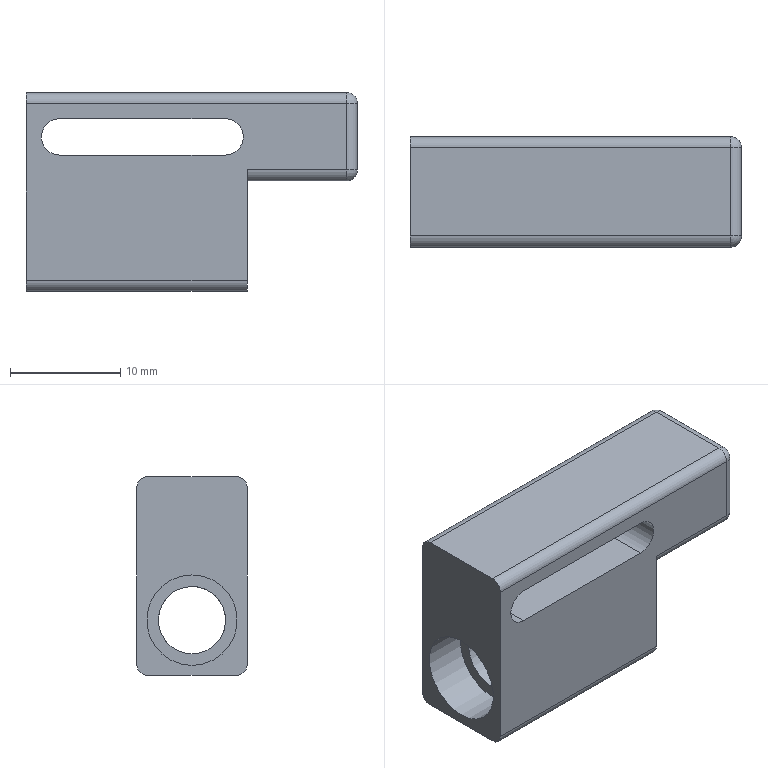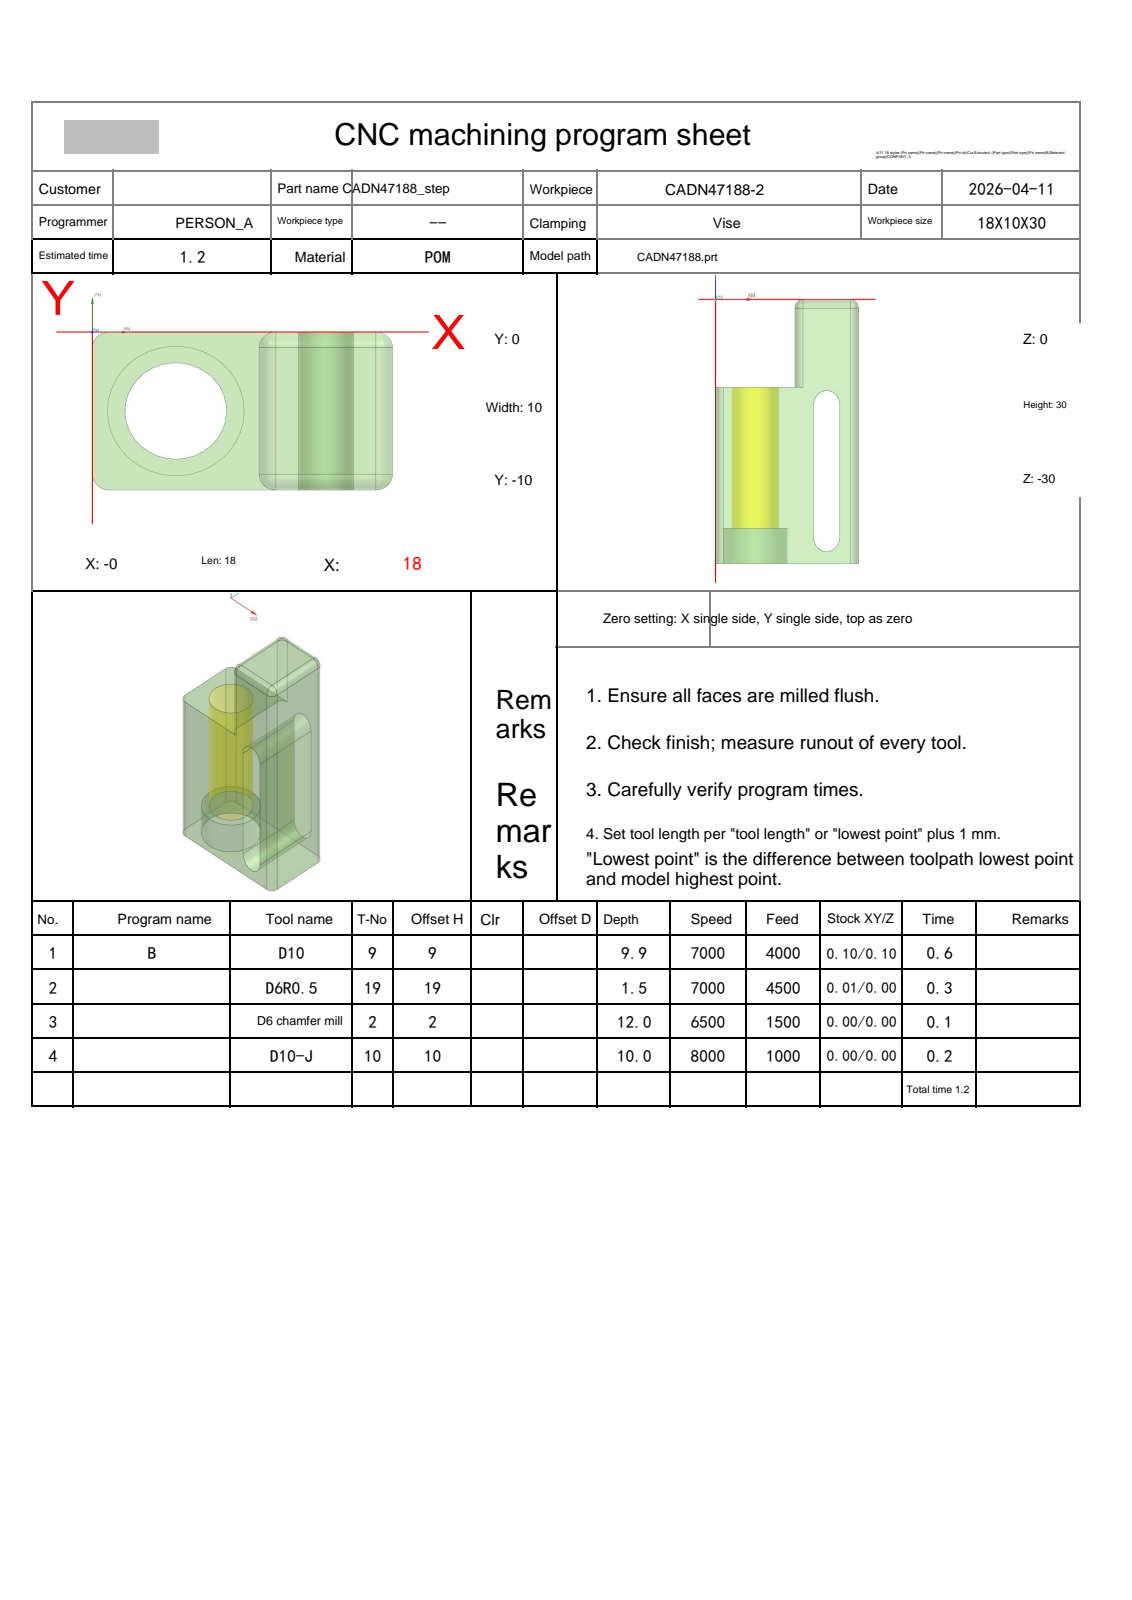NC program | NX | posted by the shop | part box 30 x 10 x 18 mm
Lines 3871 to 3974 of 3974:
N3 T02 M06
(D6 chamfer mill  D=6. R=0. H=02 ce=0.00 di=0.00)
G00 G90 G54 X8.028 Y-11.959 M03 S6500
G43 H02 Z20.
M08
Z-2.127
G01 Z-12. F1500.
G03 X7.828 Y-11.819 I-.9 J-1.072
G01 X7.797 Y-11.795
X7.758 Y-11.8
X1.
G02 X-1.8 Y-9. I0.0 J2.8
G01 Y-1.
G02 X1. Y1.8 I2.8 J0.0
G01 X7.758
X7.797 Y1.795
X7.828 Y1.819
G03 X8.028 Y1.959 I-.7 J1.212
G01 Z-2.127
G00 Z-.75
X6.065 Y-5.407
Z-2.468
G01 Z-12.
G03 X6.234 Y-5.102 I-1.658 J1.118
G01 X6.259 Y-5.054
X6.25 Y-5.
G03 X5. Y-3.75 I-1.25 J0.0
X3.75 Y-5. I0.0 J-1.25
X5. Y-6.25 I1.25 J0.0
X6.223 Y-5.26 I0.0 J1.25
G01 X6.25 Y-5.
X6.259 Y-4.946
X6.234 Y-4.898
G03 X6.065 Y-4.593 I-1.827 J-.813
G01 Z-2.468
G00 Z20.
G91 G28 Z0.0
M05
M09
G91 G28 Z0.0
M01
N4 T10 M06
(D10-J  D=10. R=0. H=10 ce=0.00 di=0.00)
G00 G90 G54 X34.971 Y-9.996 M03 S7000
G43 H10 Z20.
M08
Z2.
G01 Z0.0 F1000.
X22.916 Y-9.997
X-4.098 Y-9.998
G02 X-4.998 Y-9.116 I0.0 J.9
G01 X-4.999 Y-9.
Y-5.001
G02 X-3.999 Y-4.001 I1. J0.0
G01 X22.999 Y-4.
X34.999 Y-3.999
Z2.
G00 Z20.
G00 G90 X-5.762 Y3.275 M03 S8000
Z14.8
Z-8.5
G01 Z-10. F1000.
X-2.013 Y2.771
G02 X-.28 Y.789 I-.267 J-1.982
X-.298 Y.522 I-2. J0.0
G03 X-.4 Y-1. I11.298 J-1.522
G01 Y-9.
G03 X-.354 Y-10.024 I11.4 J0.0
X.284 Y-10.867 I.996 J.09
X1. Y-11. I.716 J1.867
G01 X3.539 Y-12.215
G03 X3.971 Y-12.313 I.432 J.902
X4.971 Y-11.313 I0.0 J1.
X4.921 Y-11. I-1. J0.0
G02 X4.6 Y-9. I6.079 J2.
G01 Y-1.
G02 X4.921 Y1. I6.4 J0.0
G03 X5.021 Y1.625 I-1.9 J.625
X3.646 Y3.525 I-2. J0.0
G01 X-3.234 Y5.788
Z-8.5
G00 Z14.8
G00 G90 X12.747 Y-17.2 M03 S8000
Z14.8
Z-9.
G01 Z-10. F1000.
G41 D10
Y-17.
Y-16.996
G03 X10.81 Y-14.997 I-2. J0.0
G02 X5. Y-9. I.19 J5.997
G01 Y-1.
G02 X10.81 Y4.997 I6. J0.0
G03 X12.747 Y6.996 I-.063 J1.999
G01 Y7.
G40 Y7.2
Z-9.
G00 Z14.8
M05
M09
G91 G28 Z0.0
G91 G28 Y0.0
M30
%